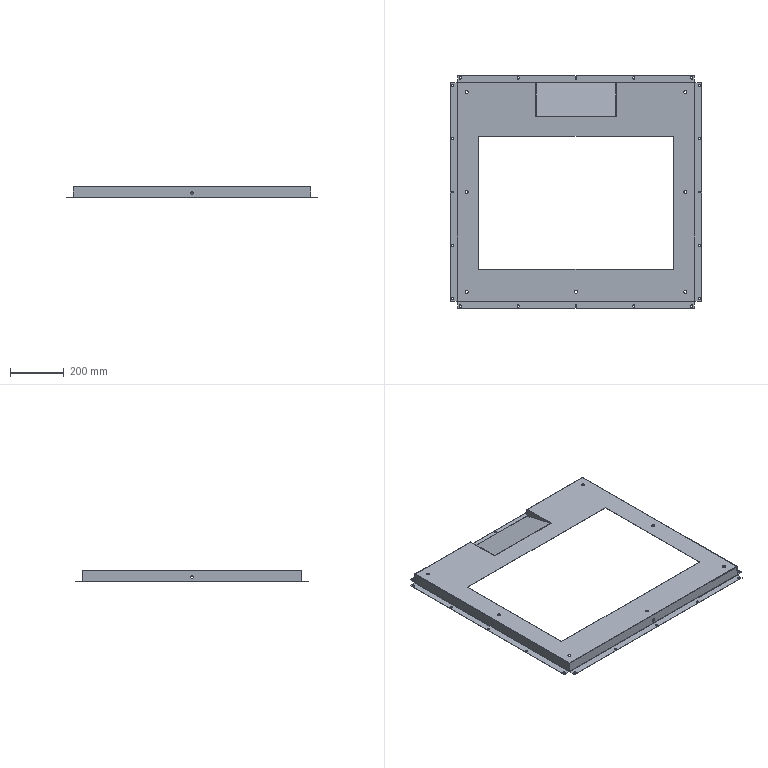Part | 2 solids | 214 faces | box 939 x 869 x 40 mm | volume 575544 mm3 | plane 110 | cylinder 92 | spline 12 | commonest cylinder face diameters 7 x50 11 x14 0.4 x11 2.4 x11 10 x6